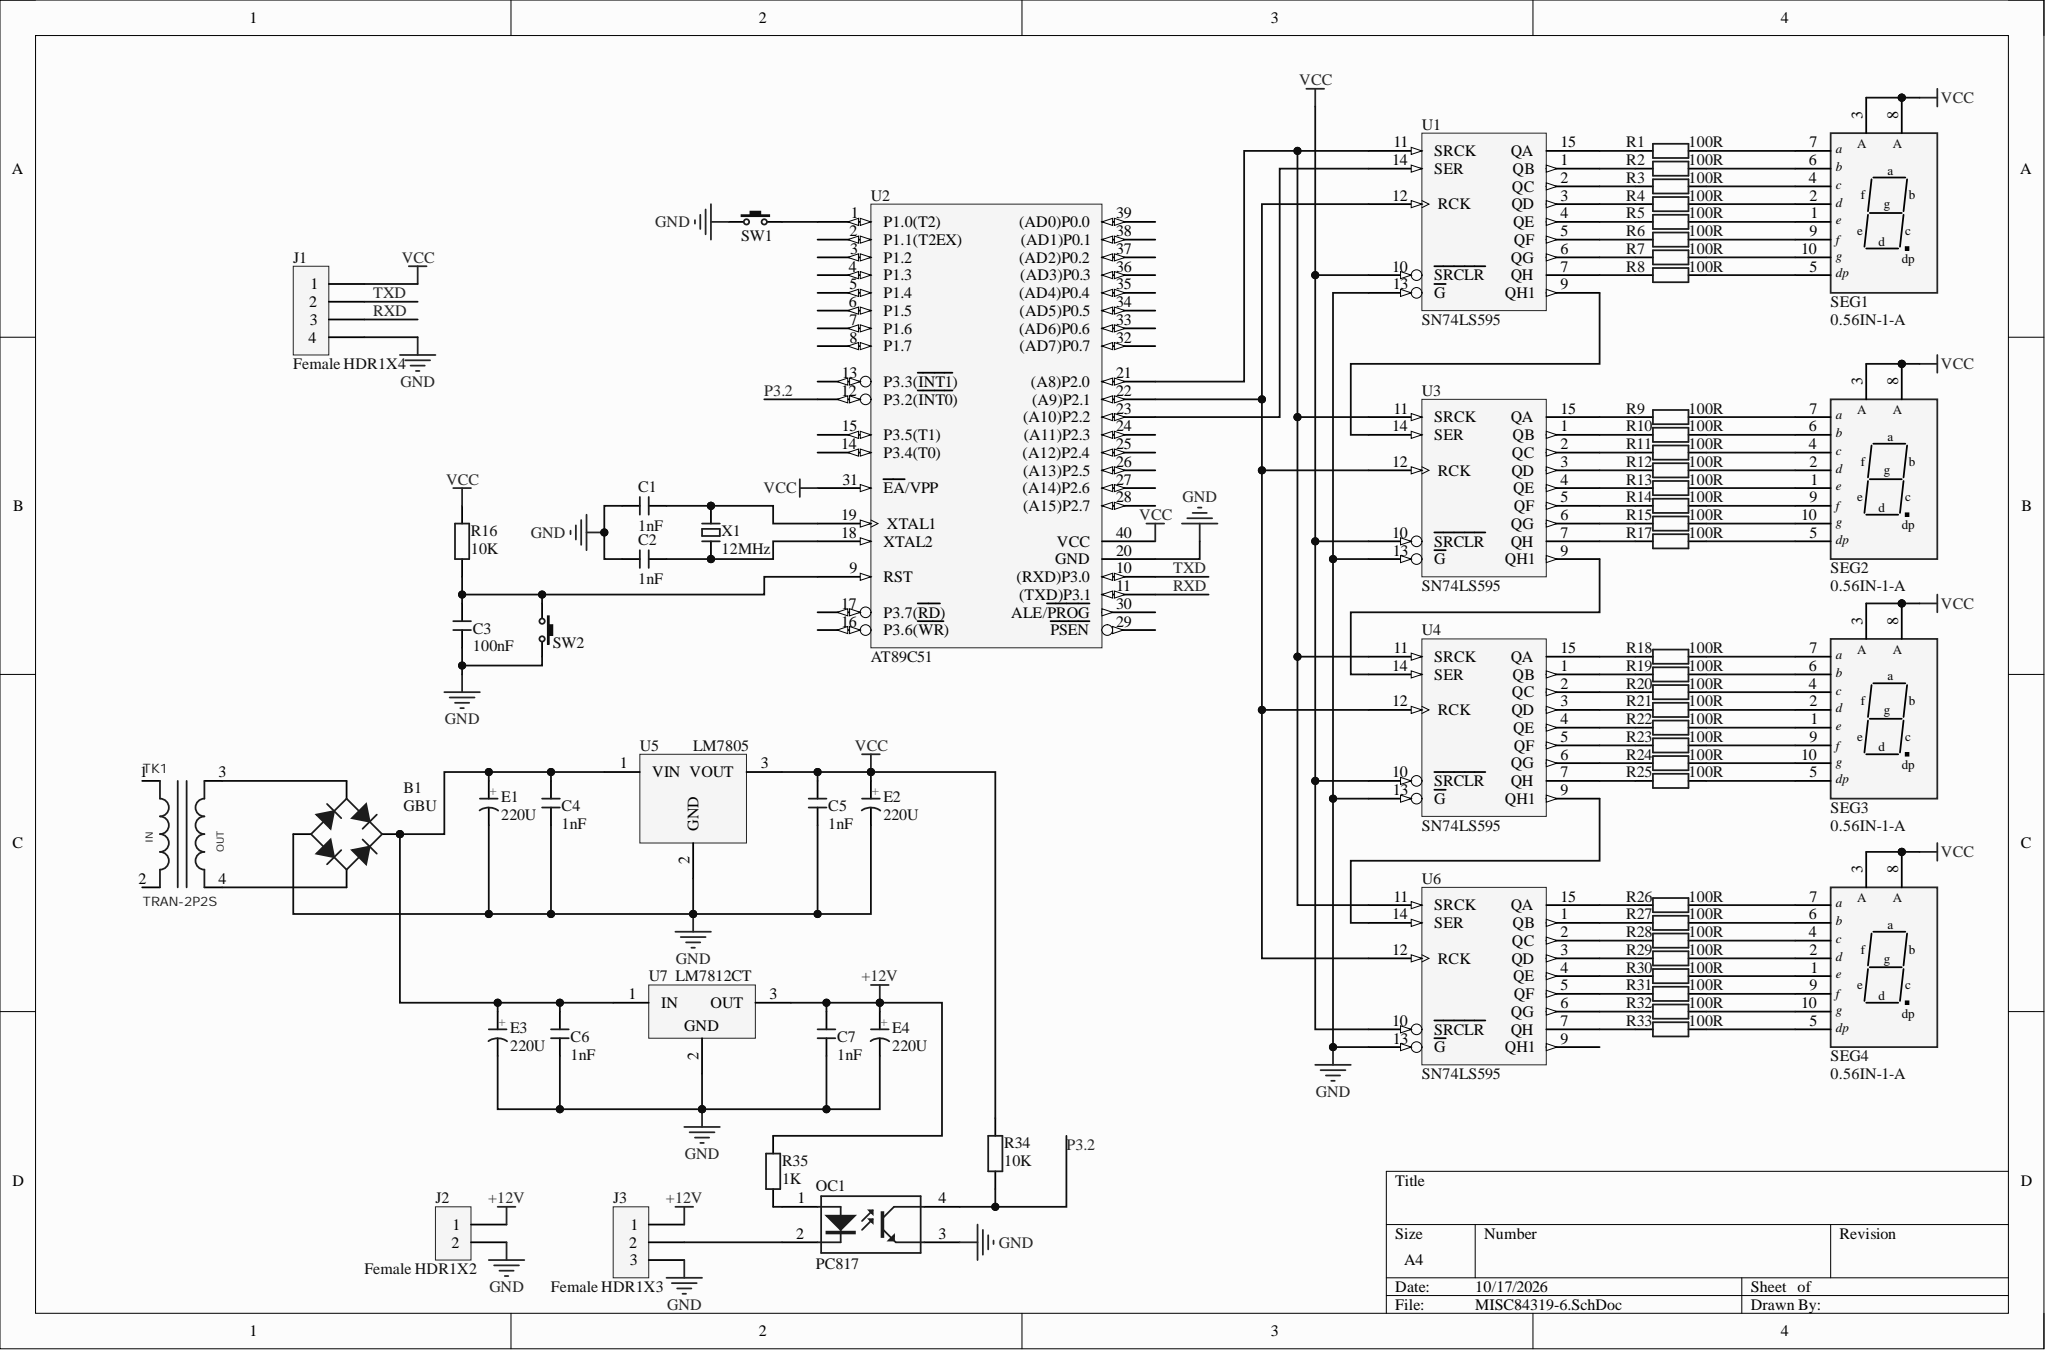Circuit board | Altium Designer | 66 parts | 85 nets
Bill of materials:
Comment,Description,Designator,Footprint,LibRef,Quantity
"GBU","1kV/10A bridge rectifier","B1","GBU","GBU","1"
"1nF","ceramic disc capacitor","C1, C2, C4, C5, C6, C7","CC 1.8*3.6","CC","6"
"100nF","ceramic disc capacitor","C3","CC 1.8*3.6","CC","1"
"220U","through-hole solid-state capacitor","E1, E2, E3, E4","CS 2.0*5*8 - C","CS","4"
"Female HDR1X4","","J1","Fe-HDR1X4/2.54-S","Female HDR1X4","1"
"Female HDR1X2","","J2","Fe-HDR1X2/2.54-S","Female HDR1X2","1"
"Female HDR1X3","","J3","Fe-HDR1X3/2.54-S","Female HDR1X3","1"
"PC817","linear optocoupler","OC1","DIP_PC817","PC817","1"
"100R","colour-band resistor","R1, R2, R3, R4, R5, R6, R7, R8, R9, R10, R11, R12, R13, R14, R15, R17, R18, R19, R20, R21, R22, R23, R24, R25, R26, R27, R28, R29, R30, R31, R32, R33","RS 1/4W","R-S","32"
"10K","colour-band resistor","R16, R34","RS 1/4W","R-S","2"
"1K","colour-band resistor","R35","RS 1/4W","R-S","1"
"0.56IN-1-A","1-digit 0.56 inch common-anode display","SEG1, SEG2, SEG3, SEG4","0.56IN-1P","0.56IN-1-A","4"
"3x6x5","3x6 tact switch","SW1, SW2","TSW DIP-3*6*5","TSW 3x6","2"
"TRAN-2P2S","","TK1","TRANS2P2S","TRAN-2P2S","1"
"SN74LS595","8-BIT SFT REG WIRTH OUTPUT LCH","U1, U3, U4, U6","DIP-16","SN74LS595","4"
"AT89C51","","U2","DIP40","STC89C51","1"
"LM7805","","U5","TO220A","LM7805","1"
"LM7812CT","Series 3-Terminal Positive Regulator","U7","T03B","LM7812CT","1"
"12MHz","2-pin passive crystal oscillator","X1","OSC HC-49S","XTAL-2P","1"
Netlist (Protel format):
[
B1
GBU
GBU



]
[
C1
CC 1.8*3.6
1nF



]
[
C2
CC 1.8*3.6
1nF



]
[
C3
CC 1.8*3.6
100nF



]
[
C4
CC 1.8*3.6
1nF



]
[
C5
CC 1.8*3.6
1nF



]
[
C6
CC 1.8*3.6
1nF



]
[
C7
CC 1.8*3.6
1nF



]
[
E1
CS 2.0*5*8 - C
220U



]
[
E2
CS 2.0*5*8 - C
220U



]
[
E3
CS 2.0*5*8 - C
220U



]
[
E4
CS 2.0*5*8 - C
220U



]
[
J1
Fe-HDR1X4/2.54-S
Female HDR1X4



]
[
J2
Fe-HDR1X2/2.54-S
Female HDR1X2



]
[
J3
Fe-HDR1X3/2.54-S
Female HDR1X3



]
[
OC1
DIP_PC817
PC817



]
[
R1
RS 1/4W
100R



]
[
R2
RS 1/4W
100R



]
[
R3
RS 1/4W
100R



]
[
R4
RS 1/4W
100R



]
[
R5
RS 1/4W
100R



]
[
R6
RS 1/4W
100R



]
[
R7
RS 1/4W
100R



]
[
R8
RS 1/4W
100R



]
[
R9
RS 1/4W
100R



]
[
R10
RS 1/4W
100R



]
[
R11
RS 1/4W
100R



]
[
R12
RS 1/4W
100R



]
[
R13
RS 1/4W
100R



]
[
R14
RS 1/4W
100R



]
[
R15
RS 1/4W
100R



]
[
R16
RS 1/4W
10K



]
[
R17
RS 1/4W
100R



]
[
R18
RS 1/4W
100R



]
[
R19
RS 1/4W
100R



]
[
R20
RS 1/4W
100R



]
[
R21
RS 1/4W
100R



]
[
R22
RS 1/4W
100R



]
[
R23
RS 1/4W
100R



]
[
R24
RS 1/4W
100R



]
[
R25
RS 1/4W
100R



]
[
R26
RS 1/4W
100R



]
[
R27
RS 1/4W
100R



]
[
R28
RS 1/4W
100R



]
[
R29
RS 1/4W
100R



]
[
R30
RS 1/4W
100R



]
[
R31
RS 1/4W
100R



]
[
R32
RS 1/4W
100R



]
[
R33
RS 1/4W
100R



]
[
R34
RS 1/4W
10K



]
[
R35
RS 1/4W
1K



]
[
SEG1
0.56IN-1P
0.56IN-1-A



]
[
SEG2
0.56IN-1P
0.56IN-1-A



]
[
SEG3
0.56IN-1P
0.56IN-1-A



]
[
SEG4
0.56IN-1P
0.56IN-1-A



]
[
SW1
TSW DIP-3*6*5
3x6x5



]
[
SW2
TSW DIP-3*6*5
3x6x5



]
[
TK1
TRANS2P2S
TRAN-2P2S



]
[
U1
DIP-16
SN74LS595



]
[
U2
DIP40
AT89C51



]
[
U3
DIP-16
SN74LS595



]
[
U4
DIP-16
SN74LS595



]
[
U5
TO220A
LM7805



]
[
U6
DIP-16
SN74LS595



]
[
U7
T03B
LM7812CT



]
[
X1
OSC HC-49S
12MHz



]
(
VCC
C5-2
E2-1
J1-1
R16-2
R34-2
SEG1-3
SEG1-8
SEG2-3
SEG2-8
SEG3-3
SEG3-8
SEG4-3
SEG4-8
U1-10
U1-16
U2-31
U2-40
U3-10
U3-16
U4-10
U4-16
U5-3
U6-10
U6-16
)
(
TXD
J1-2
U2-10
)
(
RXD
J1-3
U2-11
)
(
P3.2
OC1-4
R34-1
U2-12
)
(
NetU4_9
U4-9
U6-14
)
(
NetU3_9
U3-9
U4-14
)
(
NetU1_14
U1-14
U2-23
)
(
NetU1_12
U1-12
U2-22
U3-12
U4-12
U6-12
)
(
NetU1_11
U1-11
U2-21
U3-11
U4-11
U6-11
)
(
NetU1_9
U1-9
U3-14
)
(
NetSW1_2
SW1-2
U2-1
)
(
NetR33_2
R33-2
SEG4-5
)
(
NetR33_1
R33-1
U6-7
)
(
NetR32_2
R32-2
SEG4-10
)
(
NetR32_1
R32-1
U6-6
)
(
NetR31_2
R31-2
SEG4-9
)
(
NetR31_1
R31-1
U6-5
)
(
NetR30_2
R30-2
SEG4-1
)
(
NetR30_1
R30-1
U6-4
)
(
NetR29_2
R29-2
SEG4-2
)
(
NetR29_1
R29-1
U6-3
)
(
NetR28_2
R28-2
SEG4-4
)
(
NetR28_1
R28-1
U6-2
)
(
NetR27_2
R27-2
SEG4-6
)
(
NetR27_1
R27-1
U6-1
)
(
NetR26_2
R26-2
SEG4-7
)
(
NetR26_1
R26-1
U6-15
)
(
NetR25_2
R25-2
SEG3-5
)
(
NetR25_1
R25-1
U4-7
)
(
NetR24_2
R24-2
SEG3-10
)
(
NetR24_1
R24-1
U4-6
)
(
NetR23_2
R23-2
SEG3-9
)
(
NetR23_1
R23-1
U4-5
)
(
NetR22_2
R22-2
SEG3-1
)
(
NetR22_1
R22-1
U4-4
)
(
NetR21_2
R21-2
SEG3-2
)
(
NetR21_1
R21-1
U4-3
)
(
NetR20_2
R20-2
SEG3-4
)
(
NetR20_1
R20-1
U4-2
)
(
NetR19_2
R19-2
SEG3-6
)
(
NetR19_1
R19-1
U4-1
)
(
NetR18_2
R18-2
SEG3-7
)
(
NetR18_1
R18-1
U4-15
)
(
NetR17_2
R17-2
SEG2-5
)
(
NetR17_1
R17-1
U3-7
)
(
NetR15_2
R15-2
SEG2-10
)
(
NetR15_1
R15-1
U3-6
)
(
NetR14_2
R14-2
SEG2-9
)
(
NetR14_1
R14-1
U3-5
)
(
NetR13_2
R13-2
SEG2-1
)
(
NetR13_1
R13-1
U3-4
)
(
NetR12_2
R12-2
SEG2-2
)
(
NetR12_1
R12-1
U3-3
)
(
NetR11_2
R11-2
SEG2-4
)
(
NetR11_1
R11-1
U3-2
)
(
NetR10_2
R10-2
SEG2-6
)
(
NetR10_1
R10-1
U3-1
)
(
NetR9_2
R9-2
SEG2-7
)
(
NetR9_1
R9-1
U3-15
)
(
NetR8_2
R8-2
SEG1-5
)
(
NetR8_1
R8-1
U1-7
)
(
NetR7_2
R7-2
SEG1-10
)
(
NetR7_1
R7-1
U1-6
)
(
NetR6_2
R6-2
SEG1-9
)
(
NetR6_1
R6-1
U1-5
)
(
NetR5_2
R5-2
SEG1-1
)
(
NetR5_1
R5-1
U1-4
)
(
NetR4_2
R4-2
SEG1-2
)
(
NetR4_1
R4-1
U1-3
)
(
NetR3_2
R3-2
SEG1-4
)
(
NetR3_1
R3-1
U1-2
)
(
NetR2_2
R2-2
SEG1-6
)
(
NetR2_1
R2-1
U1-1
)
(
NetR1_2
R1-2
SEG1-7
)
(
NetR1_1
R1-1
U1-15
)
(
NetOC1_1
OC1-1
R35-1
)
(
NetJ3_2
J3-2
OC1-2
)
(
NetC3_2
C3-2
R16-1
SW2-1
U2-9
)
(
NetC2_2
C2-2
U2-18
X1-1
)
(
NetC1_2
C1-2
U2-19
X1-2
)
(
NetB1_DC+
B1-DC+
C4-2
C6-2
E1-1
E3-1
U5-1
U7-1
)
(
NetB1_AC2
B1-AC2
TK1-4
)
(
NetB1_AC1
B1-AC1
TK1-3
)
(
GND
B1-DC-
C1-1
C2-1
C3-1
C4-1
C5-1
C6-1
C7-1
E1-2
E2-2
E3-2
E4-2
J1-4
J2-2
J3-3
OC1-3
SW1-1
SW2-2
U1-8
U1-13
U2-20
U3-8
U3-13
U4-8
U4-13
U5-2
U6-8
U6-13
U7-2
)
(
+12V
C7-2
E4-1
J2-1
J3-1
R35-2
U7-3
)